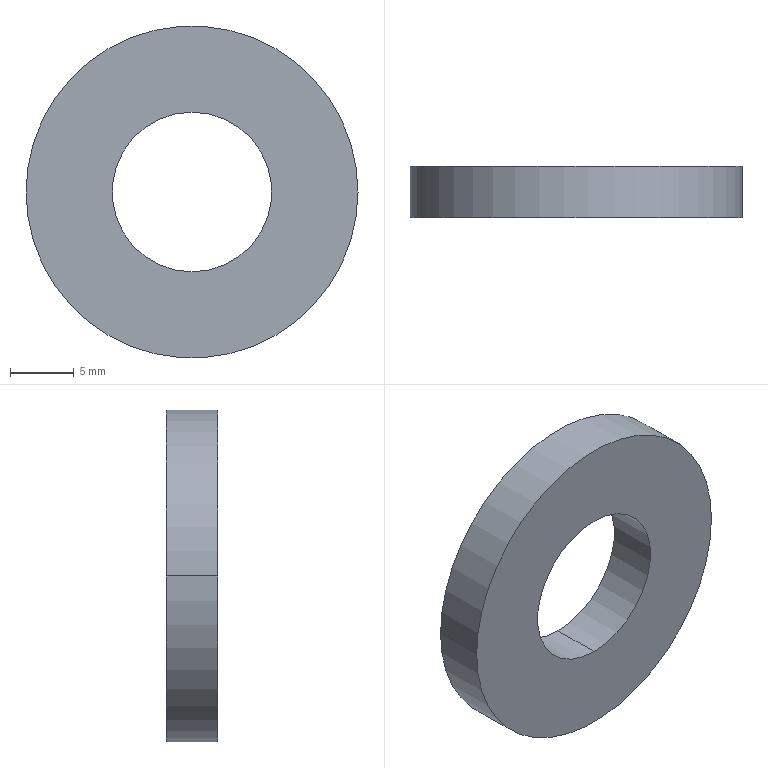Part | STEP file | WSX-SUS-M12X26-4 | 1 solid | 6 faces | box 26 x 4 x 26 mm | volume 1633 mm3 | cylinder 4 | plane 2 | commonest cylinder face diameters 12.5 x2 26 x2
STEP:
#1=CARTESIAN_POINT('',(0.,0.,0.));
#2=DIRECTION('',(0.,0.,1.));
#3=DIRECTION('',(1.,0.,0.));
#4=AXIS2_PLACEMENT_3D('',#1,#2,#3);
#5=CARTESIAN_POINT('',(0.,0.,-6.25));
#6=VERTEX_POINT('',#5);
#7=CARTESIAN_POINT('',(0.,4.,-6.25));
#8=VERTEX_POINT('',#7);
#9=CARTESIAN_POINT('',(0.,0.,-6.25));
#10=DIRECTION('',(0.,1.,0.));
#11=VECTOR('',#10,1.);
#12=LINE('',#9,#11);
#13=CARTESIAN_POINT('',(0.,0.,0.));
#14=DIRECTION('',(0.,1.,0.));
#15=DIRECTION('',(0.,0.,-1.));
#16=AXIS2_PLACEMENT_3D('',#13,#14,#15);
#17=CYLINDRICAL_SURFACE('',#16,6.25);
#18=CARTESIAN_POINT('',(6.283,0.));
#19=DIRECTION('',(0.,1.));
#20=VECTOR('',#19,1.);
#21=LINE('',#18,#20);
#22=(GEOMETRIC_REPRESENTATION_CONTEXT(2)PARAMETRIC_REPRESENTATION_CONTEXT()REPRESENTATION_CONTEXT('',''));
#23=DEFINITIONAL_REPRESENTATION('',(#21),#22);
#24=PCURVE('',#17,#23);
#25=CARTESIAN_POINT('',(0.,0.,0.));
#26=DIRECTION('',(0.,1.,0.));
#27=DIRECTION('',(0.,0.,-1.));
#28=AXIS2_PLACEMENT_3D('',#25,#26,#27);
#29=CYLINDRICAL_SURFACE('',#28,6.25);
#30=CARTESIAN_POINT('',(0.,0.));
#31=DIRECTION('',(0.,1.));
#32=VECTOR('',#31,1.);
#33=LINE('',#30,#32);
#34=(GEOMETRIC_REPRESENTATION_CONTEXT(2)PARAMETRIC_REPRESENTATION_CONTEXT()REPRESENTATION_CONTEXT('',''));
#35=DEFINITIONAL_REPRESENTATION('',(#33),#34);
#36=PCURVE('',#29,#35);
#37=SURFACE_CURVE('',#12,(#24,#36),.PCURVE_S1.);
#38=EDGE_CURVE('',#6,#8,#37,.T.);
#39=ORIENTED_EDGE('',*,*,#38,.T.);
#40=CARTESIAN_POINT('',(0.,4.,6.25));
#41=VERTEX_POINT('',#40);
#42=CARTESIAN_POINT('',(0.,4.,0.));
#43=DIRECTION('',(0.,-1.,0.));
#44=DIRECTION('',(0.,0.,1.));
#45=AXIS2_PLACEMENT_3D('',#42,#43,#44);
#46=CIRCLE('',#45,6.25);
#47=CARTESIAN_POINT('',(9.425,4.));
#48=DIRECTION('',(-1.,0.));
#49=VECTOR('',#48,1.);
#50=LINE('',#47,#49);
#51=(GEOMETRIC_REPRESENTATION_CONTEXT(2)PARAMETRIC_REPRESENTATION_CONTEXT()REPRESENTATION_CONTEXT('',''));
#52=DEFINITIONAL_REPRESENTATION('',(#50),#51);
#53=PCURVE('',#17,#52);
#54=CARTESIAN_POINT('',(0.,4.,0.));
#55=DIRECTION('',(0.,1.,0.));
#56=DIRECTION('',(-1.,0.,0.));
#57=AXIS2_PLACEMENT_3D('',#54,#55,#56);
#58=PLANE('',#57);
#59=CARTESIAN_POINT('',(0.,6.25));
#60=CARTESIAN_POINT('',(10.825,6.25));
#61=CARTESIAN_POINT('',(5.413,-3.125));
#62=CARTESIAN_POINT('',(0.,-12.5));
#63=CARTESIAN_POINT('',(-5.413,-3.125));
#64=CARTESIAN_POINT('',(-10.825,6.25));
#65=CARTESIAN_POINT('',(0.,6.25));
#66=(BOUNDED_CURVE()B_SPLINE_CURVE(2,(#59,#60,#61,#62,#63,#64,#65),.UNSPECIFIED.,.T.,.F.)B_SPLINE_CURVE_WITH_KNOTS((1,2,2,2,2,1),(-2.094,0.,2.094,4.189,6.283,8.378),.UNSPECIFIED.)CURVE()GEOMETRIC_REPRESENTATION_ITEM()RATIONAL_B_SPLINE_CURVE((1.,0.5,1.,0.5,1.,0.5,1.))REPRESENTATION_ITEM(''));
#67=(GEOMETRIC_REPRESENTATION_CONTEXT(2)PARAMETRIC_REPRESENTATION_CONTEXT()REPRESENTATION_CONTEXT('',''));
#68=DEFINITIONAL_REPRESENTATION('',(#66),#67);
#69=PCURVE('',#58,#68);
#70=SURFACE_CURVE('',#46,(#53,#69),.PCURVE_S1.);
#71=EDGE_CURVE('',#8,#41,#70,.T.);
#72=ORIENTED_EDGE('',*,*,#71,.T.);
#73=CARTESIAN_POINT('',(0.,0.,6.25));
#74=VERTEX_POINT('',#73);
#75=CARTESIAN_POINT('',(0.,0.,6.25));
#76=DIRECTION('',(0.,1.,0.));
#77=VECTOR('',#76,1.);
#78=LINE('',#75,#77);
#79=CARTESIAN_POINT('',(3.142,0.));
#80=DIRECTION('',(0.,1.));
#81=VECTOR('',#80,1.);
#82=LINE('',#79,#81);
#83=(GEOMETRIC_REPRESENTATION_CONTEXT(2)PARAMETRIC_REPRESENTATION_CONTEXT()REPRESENTATION_CONTEXT('',''));
#84=DEFINITIONAL_REPRESENTATION('',(#82),#83);
#85=PCURVE('',#17,#84);
#86=CARTESIAN_POINT('',(3.142,0.));
#87=DIRECTION('',(0.,1.));
#88=VECTOR('',#87,1.);
#89=LINE('',#86,#88);
#90=(GEOMETRIC_REPRESENTATION_CONTEXT(2)PARAMETRIC_REPRESENTATION_CONTEXT()REPRESENTATION_CONTEXT('',''));
#91=DEFINITIONAL_REPRESENTATION('',(#89),#90);
#92=PCURVE('',#29,#91);
#93=SURFACE_CURVE('',#78,(#85,#92),.PCURVE_S1.);
#94=EDGE_CURVE('',#74,#41,#93,.T.);
#95=ORIENTED_EDGE('',*,*,#94,.F.);
#96=CARTESIAN_POINT('',(0.,0.,0.));
#97=DIRECTION('',(0.,1.,0.));
#98=DIRECTION('',(0.,0.,-1.));
#99=AXIS2_PLACEMENT_3D('',#96,#97,#98);
#100=CIRCLE('',#99,6.25);
#101=CARTESIAN_POINT('',(0.,0.));
#102=DIRECTION('',(1.,0.));
#103=VECTOR('',#102,1.);
#104=LINE('',#101,#103);
#105=(GEOMETRIC_REPRESENTATION_CONTEXT(2)PARAMETRIC_REPRESENTATION_CONTEXT()REPRESENTATION_CONTEXT('',''));
#106=DEFINITIONAL_REPRESENTATION('',(#104),#105);
#107=PCURVE('',#17,#106);
#108=CARTESIAN_POINT('',(0.,0.,0.));
#109=DIRECTION('',(0.,-1.,0.));
#110=DIRECTION('',(1.,0.,0.));
#111=AXIS2_PLACEMENT_3D('',#108,#109,#110);
#112=PLANE('',#111);
#113=CARTESIAN_POINT('',(0.,-6.25));
#114=CARTESIAN_POINT('',(-10.825,-6.25));
#115=CARTESIAN_POINT('',(-5.413,3.125));
#116=CARTESIAN_POINT('',(0.,12.5));
#117=CARTESIAN_POINT('',(5.413,3.125));
#118=CARTESIAN_POINT('',(10.825,-6.25));
#119=CARTESIAN_POINT('',(0.,-6.25));
#120=(BOUNDED_CURVE()B_SPLINE_CURVE(2,(#113,#114,#115,#116,#117,#118,#119),.UNSPECIFIED.,.T.,.F.)B_SPLINE_CURVE_WITH_KNOTS((1,2,2,2,2,1),(-2.094,0.,2.094,4.189,6.283,8.378),.UNSPECIFIED.)CURVE()GEOMETRIC_REPRESENTATION_ITEM()RATIONAL_B_SPLINE_CURVE((1.,0.5,1.,0.5,1.,0.5,1.))REPRESENTATION_ITEM(''));
#121=(GEOMETRIC_REPRESENTATION_CONTEXT(2)PARAMETRIC_REPRESENTATION_CONTEXT()REPRESENTATION_CONTEXT('',''));
#122=DEFINITIONAL_REPRESENTATION('',(#120),#121);
#123=PCURVE('',#112,#122);
#124=SURFACE_CURVE('',#100,(#107,#123),.PCURVE_S1.);
#125=EDGE_CURVE('',#74,#6,#124,.T.);
#126=ORIENTED_EDGE('',*,*,#125,.T.);
#127=EDGE_LOOP('',(#39,#72,#95,#126));
#128=FACE_BOUND('',#127,.F.);
#129=ADVANCED_FACE('',(#128),#17,.F.);
#130=CARTESIAN_POINT('',(-13.,0.,0.));
#131=VERTEX_POINT('',#130);
#132=CARTESIAN_POINT('',(13.,0.,0.));
#133=VERTEX_POINT('',#132);
#134=CARTESIAN_POINT('',(0.,0.,0.));
#135=DIRECTION('',(0.,1.,0.));
#136=DIRECTION('',(-1.,0.,0.));
#137=AXIS2_PLACEMENT_3D('',#134,#135,#136);
#138=CIRCLE('',#137,13.);
#139=CARTESIAN_POINT('',(0.,0.,0.));
#140=DIRECTION('',(0.,1.,0.));
#141=DIRECTION('',(-1.,0.,0.));
#142=AXIS2_PLACEMENT_3D('',#139,#140,#141);
#143=CYLINDRICAL_SURFACE('',#142,13.);
#144=CARTESIAN_POINT('',(0.,0.));
#145=DIRECTION('',(1.,0.));
#146=VECTOR('',#145,1.);
#147=LINE('',#144,#146);
#148=(GEOMETRIC_REPRESENTATION_CONTEXT(2)PARAMETRIC_REPRESENTATION_CONTEXT()REPRESENTATION_CONTEXT('',''));
#149=DEFINITIONAL_REPRESENTATION('',(#147),#148);
#150=PCURVE('',#143,#149);
#151=CARTESIAN_POINT('',(-13.,0.));
#152=CARTESIAN_POINT('',(-13.,22.517));
#153=CARTESIAN_POINT('',(6.5,11.258));
#154=CARTESIAN_POINT('',(26.,0.));
#155=CARTESIAN_POINT('',(6.5,-11.258));
#156=CARTESIAN_POINT('',(-13.,-22.517));
#157=CARTESIAN_POINT('',(-13.,0.));
#158=(BOUNDED_CURVE()B_SPLINE_CURVE(2,(#151,#152,#153,#154,#155,#156,#157),.UNSPECIFIED.,.T.,.F.)B_SPLINE_CURVE_WITH_KNOTS((1,2,2,2,2,1),(-2.094,0.,2.094,4.189,6.283,8.378),.UNSPECIFIED.)CURVE()GEOMETRIC_REPRESENTATION_ITEM()RATIONAL_B_SPLINE_CURVE((1.,0.5,1.,0.5,1.,0.5,1.))REPRESENTATION_ITEM(''));
#159=(GEOMETRIC_REPRESENTATION_CONTEXT(2)PARAMETRIC_REPRESENTATION_CONTEXT()REPRESENTATION_CONTEXT('',''));
#160=DEFINITIONAL_REPRESENTATION('',(#158),#159);
#161=PCURVE('',#112,#160);
#162=SURFACE_CURVE('',#138,(#150,#161),.PCURVE_S1.);
#163=EDGE_CURVE('',#131,#133,#162,.T.);
#164=ORIENTED_EDGE('',*,*,#163,.T.);
#165=CARTESIAN_POINT('',(13.,4.,0.));
#166=VERTEX_POINT('',#165);
#167=CARTESIAN_POINT('',(13.,0.,0.));
#168=DIRECTION('',(0.,1.,0.));
#169=VECTOR('',#168,1.);
#170=LINE('',#167,#169);
#171=CARTESIAN_POINT('',(3.142,0.));
#172=DIRECTION('',(0.,1.));
#173=VECTOR('',#172,1.);
#174=LINE('',#171,#173);
#175=(GEOMETRIC_REPRESENTATION_CONTEXT(2)PARAMETRIC_REPRESENTATION_CONTEXT()REPRESENTATION_CONTEXT('',''));
#176=DEFINITIONAL_REPRESENTATION('',(#174),#175);
#177=PCURVE('',#143,#176);
#178=CARTESIAN_POINT('',(0.,0.,0.));
#179=DIRECTION('',(0.,1.,0.));
#180=DIRECTION('',(-1.,0.,0.));
#181=AXIS2_PLACEMENT_3D('',#178,#179,#180);
#182=CYLINDRICAL_SURFACE('',#181,13.);
#183=CARTESIAN_POINT('',(3.142,0.));
#184=DIRECTION('',(0.,1.));
#185=VECTOR('',#184,1.);
#186=LINE('',#183,#185);
#187=(GEOMETRIC_REPRESENTATION_CONTEXT(2)PARAMETRIC_REPRESENTATION_CONTEXT()REPRESENTATION_CONTEXT('',''));
#188=DEFINITIONAL_REPRESENTATION('',(#186),#187);
#189=PCURVE('',#182,#188);
#190=SURFACE_CURVE('',#170,(#177,#189),.PCURVE_S1.);
#191=EDGE_CURVE('',#133,#166,#190,.T.);
#192=ORIENTED_EDGE('',*,*,#191,.T.);
#193=CARTESIAN_POINT('',(-13.,4.,0.));
#194=VERTEX_POINT('',#193);
#195=CARTESIAN_POINT('',(0.,4.,0.));
#196=DIRECTION('',(0.,-1.,0.));
#197=DIRECTION('',(1.,0.,0.));
#198=AXIS2_PLACEMENT_3D('',#195,#196,#197);
#199=CIRCLE('',#198,13.);
#200=CARTESIAN_POINT('',(3.142,4.));
#201=DIRECTION('',(-1.,0.));
#202=VECTOR('',#201,1.);
#203=LINE('',#200,#202);
#204=(GEOMETRIC_REPRESENTATION_CONTEXT(2)PARAMETRIC_REPRESENTATION_CONTEXT()REPRESENTATION_CONTEXT('',''));
#205=DEFINITIONAL_REPRESENTATION('',(#203),#204);
#206=PCURVE('',#143,#205);
#207=CARTESIAN_POINT('',(-13.,0.));
#208=CARTESIAN_POINT('',(-13.,22.517));
#209=CARTESIAN_POINT('',(6.5,11.258));
#210=CARTESIAN_POINT('',(26.,0.));
#211=CARTESIAN_POINT('',(6.5,-11.258));
#212=CARTESIAN_POINT('',(-13.,-22.517));
#213=CARTESIAN_POINT('',(-13.,0.));
#214=(BOUNDED_CURVE()B_SPLINE_CURVE(2,(#207,#208,#209,#210,#211,#212,#213),.UNSPECIFIED.,.T.,.F.)B_SPLINE_CURVE_WITH_KNOTS((1,2,2,2,2,1),(-2.094,0.,2.094,4.189,6.283,8.378),.UNSPECIFIED.)CURVE()GEOMETRIC_REPRESENTATION_ITEM()RATIONAL_B_SPLINE_CURVE((1.,0.5,1.,0.5,1.,0.5,1.))REPRESENTATION_ITEM(''));
#215=(GEOMETRIC_REPRESENTATION_CONTEXT(2)PARAMETRIC_REPRESENTATION_CONTEXT()REPRESENTATION_CONTEXT('',''));
#216=DEFINITIONAL_REPRESENTATION('',(#214),#215);
#217=PCURVE('',#58,#216);
#218=SURFACE_CURVE('',#199,(#206,#217),.PCURVE_S1.);
#219=EDGE_CURVE('',#166,#194,#218,.T.);
#220=ORIENTED_EDGE('',*,*,#219,.T.);
#221=CARTESIAN_POINT('',(-13.,0.,0.));
#222=DIRECTION('',(0.,1.,0.));
#223=VECTOR('',#222,1.);
#224=LINE('',#221,#223);
#225=CARTESIAN_POINT('',(0.,0.));
#226=DIRECTION('',(0.,1.));
#227=VECTOR('',#226,1.);
#228=LINE('',#225,#227);
#229=(GEOMETRIC_REPRESENTATION_CONTEXT(2)PARAMETRIC_REPRESENTATION_CONTEXT()REPRESENTATION_CONTEXT('',''));
#230=DEFINITIONAL_REPRESENTATION('',(#228),#229);
#231=PCURVE('',#143,#230);
#232=CARTESIAN_POINT('',(6.283,0.));
#233=DIRECTION('',(0.,1.));
#234=VECTOR('',#233,1.);
#235=LINE('',#232,#234);
#236=(GEOMETRIC_REPRESENTATION_CONTEXT(2)PARAMETRIC_REPRESENTATION_CONTEXT()REPRESENTATION_CONTEXT('',''));
#237=DEFINITIONAL_REPRESENTATION('',(#235),#236);
#238=PCURVE('',#182,#237);
#239=SURFACE_CURVE('',#224,(#231,#238),.PCURVE_S1.);
#240=EDGE_CURVE('',#131,#194,#239,.T.);
#241=ORIENTED_EDGE('',*,*,#240,.F.);
#242=EDGE_LOOP('',(#164,#192,#220,#241));
#243=FACE_BOUND('',#242,.T.);
#244=ADVANCED_FACE('',(#243),#143,.T.);
#245=ORIENTED_EDGE('',*,*,#71,.T.);
#246=CARTESIAN_POINT('',(0.,4.,0.));
#247=DIRECTION('',(0.,-1.,0.));
#248=DIRECTION('',(0.,0.,1.));
#249=AXIS2_PLACEMENT_3D('',#246,#247,#248);
#250=CIRCLE('',#249,6.25);
#251=CARTESIAN_POINT('',(0.,6.25));
#252=CARTESIAN_POINT('',(10.825,6.25));
#253=CARTESIAN_POINT('',(5.413,-3.125));
#254=CARTESIAN_POINT('',(0.,-12.5));
#255=CARTESIAN_POINT('',(-5.413,-3.125));
#256=CARTESIAN_POINT('',(-10.825,6.25));
#257=CARTESIAN_POINT('',(0.,6.25));
#258=(BOUNDED_CURVE()B_SPLINE_CURVE(2,(#251,#252,#253,#254,#255,#256,#257),.UNSPECIFIED.,.T.,.F.)B_SPLINE_CURVE_WITH_KNOTS((1,2,2,2,2,1),(-2.094,0.,2.094,4.189,6.283,8.378),.UNSPECIFIED.)CURVE()GEOMETRIC_REPRESENTATION_ITEM()RATIONAL_B_SPLINE_CURVE((1.,0.5,1.,0.5,1.,0.5,1.))REPRESENTATION_ITEM(''));
#259=(GEOMETRIC_REPRESENTATION_CONTEXT(2)PARAMETRIC_REPRESENTATION_CONTEXT()REPRESENTATION_CONTEXT('',''));
#260=DEFINITIONAL_REPRESENTATION('',(#258),#259);
#261=PCURVE('',#58,#260);
#262=CARTESIAN_POINT('',(3.142,4.));
#263=DIRECTION('',(-1.,0.));
#264=VECTOR('',#263,1.);
#265=LINE('',#262,#264);
#266=(GEOMETRIC_REPRESENTATION_CONTEXT(2)PARAMETRIC_REPRESENTATION_CONTEXT()REPRESENTATION_CONTEXT('',''));
#267=DEFINITIONAL_REPRESENTATION('',(#265),#266);
#268=PCURVE('',#29,#267);
#269=SURFACE_CURVE('',#250,(#261,#268),.PCURVE_S1.);
#270=EDGE_CURVE('',#41,#8,#269,.T.);
#271=ORIENTED_EDGE('',*,*,#270,.T.);
#272=EDGE_LOOP('',(#245,#271));
#273=FACE_BOUND('',#272,.T.);
#274=CARTESIAN_POINT('',(0.,4.,0.));
#275=DIRECTION('',(0.,-1.,0.));
#276=DIRECTION('',(1.,0.,0.));
#277=AXIS2_PLACEMENT_3D('',#274,#275,#276);
#278=CIRCLE('',#277,13.);
#279=CARTESIAN_POINT('',(-13.,0.));
#280=CARTESIAN_POINT('',(-13.,22.517));
#281=CARTESIAN_POINT('',(6.5,11.258));
#282=CARTESIAN_POINT('',(26.,0.));
#283=CARTESIAN_POINT('',(6.5,-11.258));
#284=CARTESIAN_POINT('',(-13.,-22.517));
#285=CARTESIAN_POINT('',(-13.,0.));
#286=(BOUNDED_CURVE()B_SPLINE_CURVE(2,(#279,#280,#281,#282,#283,#284,#285),.UNSPECIFIED.,.T.,.F.)B_SPLINE_CURVE_WITH_KNOTS((1,2,2,2,2,1),(-2.094,0.,2.094,4.189,6.283,8.378),.UNSPECIFIED.)CURVE()GEOMETRIC_REPRESENTATION_ITEM()RATIONAL_B_SPLINE_CURVE((1.,0.5,1.,0.5,1.,0.5,1.))REPRESENTATION_ITEM(''));
#287=(GEOMETRIC_REPRESENTATION_CONTEXT(2)PARAMETRIC_REPRESENTATION_CONTEXT()REPRESENTATION_CONTEXT('',''));
#288=DEFINITIONAL_REPRESENTATION('',(#286),#287);
#289=PCURVE('',#58,#288);
#290=CARTESIAN_POINT('',(9.425,4.));
#291=DIRECTION('',(-1.,0.));
#292=VECTOR('',#291,1.);
#293=LINE('',#290,#292);
#294=(GEOMETRIC_REPRESENTATION_CONTEXT(2)PARAMETRIC_REPRESENTATION_CONTEXT()REPRESENTATION_CONTEXT('',''));
#295=DEFINITIONAL_REPRESENTATION('',(#293),#294);
#296=PCURVE('',#182,#295);
#297=SURFACE_CURVE('',#278,(#289,#296),.PCURVE_S1.);
#298=EDGE_CURVE('',#194,#166,#297,.T.);
#299=ORIENTED_EDGE('',*,*,#298,.F.);
#300=ORIENTED_EDGE('',*,*,#219,.F.);
#301=EDGE_LOOP('',(#299,#300));
#302=FACE_BOUND('',#301,.T.);
#303=ADVANCED_FACE('',(#273,#302),#58,.T.);
#304=CARTESIAN_POINT('',(0.,0.,0.));
#305=DIRECTION('',(0.,1.,0.));
#306=DIRECTION('',(0.,0.,-1.));
#307=AXIS2_PLACEMENT_3D('',#304,#305,#306);
#308=CIRCLE('',#307,6.25);
#309=CARTESIAN_POINT('',(0.,-6.25));
#310=CARTESIAN_POINT('',(-10.825,-6.25));
#311=CARTESIAN_POINT('',(-5.413,3.125));
#312=CARTESIAN_POINT('',(0.,12.5));
#313=CARTESIAN_POINT('',(5.413,3.125));
#314=CARTESIAN_POINT('',(10.825,-6.25));
#315=CARTESIAN_POINT('',(0.,-6.25));
#316=(BOUNDED_CURVE()B_SPLINE_CURVE(2,(#309,#310,#311,#312,#313,#314,#315),.UNSPECIFIED.,.T.,.F.)B_SPLINE_CURVE_WITH_KNOTS((1,2,2,2,2,1),(-2.094,0.,2.094,4.189,6.283,8.378),.UNSPECIFIED.)CURVE()GEOMETRIC_REPRESENTATION_ITEM()RATIONAL_B_SPLINE_CURVE((1.,0.5,1.,0.5,1.,0.5,1.))REPRESENTATION_ITEM(''));
#317=(GEOMETRIC_REPRESENTATION_CONTEXT(2)PARAMETRIC_REPRESENTATION_CONTEXT()REPRESENTATION_CONTEXT('',''));
#318=DEFINITIONAL_REPRESENTATION('',(#316),#317);
#319=PCURVE('',#112,#318);
#320=CARTESIAN_POINT('',(0.,0.));
#321=DIRECTION('',(1.,0.));
#322=VECTOR('',#321,1.);
#323=LINE('',#320,#322);
#324=(GEOMETRIC_REPRESENTATION_CONTEXT(2)PARAMETRIC_REPRESENTATION_CONTEXT()REPRESENTATION_CONTEXT('',''));
#325=DEFINITIONAL_REPRESENTATION('',(#323),#324);
#326=PCURVE('',#29,#325);
#327=SURFACE_CURVE('',#308,(#319,#326),.PCURVE_S1.);
#328=EDGE_CURVE('',#6,#74,#327,.T.);
#329=ORIENTED_EDGE('',*,*,#328,.T.);
#330=ORIENTED_EDGE('',*,*,#125,.T.);
#331=EDGE_LOOP('',(#329,#330));
#332=FACE_BOUND('',#331,.T.);
#333=ORIENTED_EDGE('',*,*,#163,.F.);
#334=CARTESIAN_POINT('',(0.,0.,0.));
#335=DIRECTION('',(0.,1.,0.));
#336=DIRECTION('',(-1.,0.,0.));
#337=AXIS2_PLACEMENT_3D('',#334,#335,#336);
#338=CIRCLE('',#337,13.);
#339=CARTESIAN_POINT('',(-13.,0.));
#340=CARTESIAN_POINT('',(-13.,22.517));
#341=CARTESIAN_POINT('',(6.5,11.258));
#342=CARTESIAN_POINT('',(26.,0.));
#343=CARTESIAN_POINT('',(6.5,-11.258));
#344=CARTESIAN_POINT('',(-13.,-22.517));
#345=CARTESIAN_POINT('',(-13.,0.));
#346=(BOUNDED_CURVE()B_SPLINE_CURVE(2,(#339,#340,#341,#342,#343,#344,#345),.UNSPECIFIED.,.T.,.F.)B_SPLINE_CURVE_WITH_KNOTS((1,2,2,2,2,1),(-2.094,0.,2.094,4.189,6.283,8.378),.UNSPECIFIED.)CURVE()GEOMETRIC_REPRESENTATION_ITEM()RATIONAL_B_SPLINE_CURVE((1.,0.5,1.,0.5,1.,0.5,1.))REPRESENTATION_ITEM(''));
#347=(GEOMETRIC_REPRESENTATION_CONTEXT(2)PARAMETRIC_REPRESENTATION_CONTEXT()REPRESENTATION_CONTEXT('',''));
#348=DEFINITIONAL_REPRESENTATION('',(#346),#347);
#349=PCURVE('',#112,#348);
#350=CARTESIAN_POINT('',(0.,0.));
#351=DIRECTION('',(1.,0.));
#352=VECTOR('',#351,1.);
#353=LINE('',#350,#352);
#354=(GEOMETRIC_REPRESENTATION_CONTEXT(2)PARAMETRIC_REPRESENTATION_CONTEXT()REPRESENTATION_CONTEXT('',''));
#355=DEFINITIONAL_REPRESENTATION('',(#353),#354);
#356=PCURVE('',#182,#355);
#357=SURFACE_CURVE('',#338,(#349,#356),.PCURVE_S1.);
#358=EDGE_CURVE('',#133,#131,#357,.T.);
#359=ORIENTED_EDGE('',*,*,#358,.F.);
#360=EDGE_LOOP('',(#333,#359));
#361=FACE_BOUND('',#360,.T.);
#362=ADVANCED_FACE('',(#332,#361),#112,.T.);
#363=ORIENTED_EDGE('',*,*,#191,.F.);
#364=ORIENTED_EDGE('',*,*,#358,.T.);
#365=ORIENTED_EDGE('',*,*,#240,.T.);
#366=ORIENTED_EDGE('',*,*,#298,.T.);
#367=EDGE_LOOP('',(#363,#364,#365,#366));
#368=FACE_BOUND('',#367,.T.);
#369=ADVANCED_FACE('',(#368),#182,.T.);
#370=ORIENTED_EDGE('',*,*,#270,.T.);
#371=ORIENTED_EDGE('',*,*,#38,.F.);
#372=ORIENTED_EDGE('',*,*,#328,.T.);
#373=ORIENTED_EDGE('',*,*,#94,.T.);
#374=EDGE_LOOP('',(#370,#371,#372,#373));
#375=FACE_BOUND('',#374,.F.);
#376=ADVANCED_FACE('',(#375),#29,.F.);
#377=CLOSED_SHELL('',(#129,#244,#303,#362,#369,#376));
#378=MANIFOLD_SOLID_BREP('',#377);
#379=(LENGTH_UNIT()NAMED_UNIT(*)SI_UNIT(.MILLI.,.METRE.));
#380=UNCERTAINTY_MEASURE_WITH_UNIT(LENGTH_MEASURE(0.0000001),#379,'','');
#381=(NAMED_UNIT(*)PLANE_ANGLE_UNIT()SI_UNIT($,.RADIAN.));
#382=(NAMED_UNIT(*)SI_UNIT($,.STERADIAN.)SOLID_ANGLE_UNIT());
#383=(GEOMETRIC_REPRESENTATION_CONTEXT(3)GLOBAL_UNCERTAINTY_ASSIGNED_CONTEXT((#380))GLOBAL_UNIT_ASSIGNED_CONTEXT((#379,#381,#382))REPRESENTATION_CONTEXT('',''));
#384=ADVANCED_BREP_SHAPE_REPRESENTATION('',(#4,#378),#383);